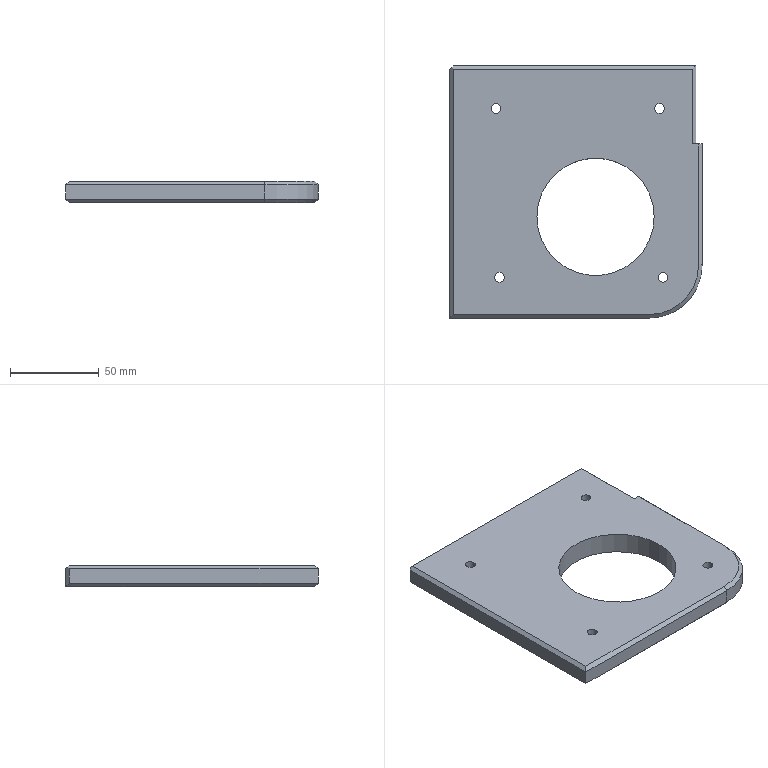Part | Creo | 1 solid | 43 faces | box 142 x 142 x 12 mm | volume 192544 mm3 | plane 22 | cylinder 19 | cone 2 | commonest cylinder face diameters 5.5 x8 9.5 x8 66 x2 60 x1
STEP:
#1=CARTESIAN_POINT('',(-313.,372.995,1.));
#2=VERTEX_POINT('',#1);
#3=CARTESIAN_POINT('',(-178.5,372.995,1.));
#4=VERTEX_POINT('',#3);
#5=CARTESIAN_POINT('',(-313.,372.995,1.));
#6=DIRECTION('',(1.,0.,0.));
#7=VECTOR('',#6,134.5);
#8=LINE('',#5,#7);
#9=EDGE_CURVE('',#2,#4,#8,.T.);
#10=ORIENTED_EDGE('',*,*,#9,.T.);
#11=CARTESIAN_POINT('',(-178.5,330.995,1.));
#12=VERTEX_POINT('',#11);
#13=CARTESIAN_POINT('',(-178.5,372.995,1.));
#14=DIRECTION('',(0.,-1.,0.));
#15=VECTOR('',#14,42.);
#16=LINE('',#13,#15);
#17=EDGE_CURVE('',#4,#12,#16,.T.);
#18=ORIENTED_EDGE('',*,*,#17,.T.);
#19=CARTESIAN_POINT('',(-175.,330.995,1.));
#20=VERTEX_POINT('',#19);
#21=CARTESIAN_POINT('',(-175.,330.995,1.));
#22=DIRECTION('',(-1.,0.,0.));
#23=VECTOR('',#22,3.5);
#24=LINE('',#21,#23);
#25=EDGE_CURVE('',#20,#12,#24,.T.);
#26=ORIENTED_EDGE('',*,*,#25,.F.);
#27=CARTESIAN_POINT('',(-175.,262.995,1.));
#28=VERTEX_POINT('',#27);
#29=CARTESIAN_POINT('',(-175.,330.995,1.));
#30=DIRECTION('',(0.,-1.,0.));
#31=VECTOR('',#30,68.);
#32=LINE('',#29,#31);
#33=EDGE_CURVE('',#20,#28,#32,.T.);
#34=ORIENTED_EDGE('',*,*,#33,.T.);
#35=CARTESIAN_POINT('',(-203.,234.995,1.));
#36=VERTEX_POINT('',#35);
#37=CARTESIAN_POINT('',(-203.,262.995,1.));
#38=DIRECTION('',(0.,0.,1.));
#39=DIRECTION('',(0.,-1.,0.));
#40=AXIS2_PLACEMENT_3D('',#37,#38,#39);
#41=CIRCLE('',#40,28.);
#42=EDGE_CURVE('',#36,#28,#41,.T.);
#43=ORIENTED_EDGE('',*,*,#42,.F.);
#44=CARTESIAN_POINT('',(-313.,234.995,1.));
#45=VERTEX_POINT('',#44);
#46=CARTESIAN_POINT('',(-203.,234.995,1.));
#47=DIRECTION('',(-1.,0.,0.));
#48=VECTOR('',#47,110.);
#49=LINE('',#46,#48);
#50=EDGE_CURVE('',#36,#45,#49,.T.);
#51=ORIENTED_EDGE('',*,*,#50,.T.);
#52=CARTESIAN_POINT('',(-313.,234.995,1.));
#53=DIRECTION('',(0.,1.,0.));
#54=VECTOR('',#53,138.);
#55=LINE('',#52,#54);
#56=EDGE_CURVE('',#45,#2,#55,.T.);
#57=ORIENTED_EDGE('',*,*,#56,.T.);
#58=EDGE_LOOP('',(#10,#18,#26,#34,#43,#51,#57));
#59=FACE_OUTER_BOUND('',#58,.F.);
#60=CARTESIAN_POINT('',(-197.75,256.,1.));
#61=VERTEX_POINT('',#60);
#62=CARTESIAN_POINT('',(-192.25,256.,1.));
#63=VERTEX_POINT('',#62);
#64=CARTESIAN_POINT('',(-195.,256.,1.));
#65=DIRECTION('',(0.,0.,-1.));
#66=DIRECTION('',(-1.,0.,0.));
#67=AXIS2_PLACEMENT_3D('',#64,#65,#66);
#68=CIRCLE('',#67,2.75);
#69=EDGE_CURVE('',#61,#63,#68,.T.);
#70=ORIENTED_EDGE('',*,*,#69,.F.);
#71=CARTESIAN_POINT('',(-195.,256.,1.));
#72=DIRECTION('',(0.,0.,-1.));
#73=DIRECTION('',(1.,0.,0.));
#74=AXIS2_PLACEMENT_3D('',#71,#72,#73);
#75=CIRCLE('',#74,2.75);
#76=EDGE_CURVE('',#63,#61,#75,.T.);
#77=ORIENTED_EDGE('',*,*,#76,.F.);
#78=EDGE_LOOP('',(#70,#77));
#79=FACE_BOUND('',#78,.F.);
#80=CARTESIAN_POINT('',(-289.75,256.,1.));
#81=VERTEX_POINT('',#80);
#82=CARTESIAN_POINT('',(-284.25,256.,1.));
#83=VERTEX_POINT('',#82);
#84=CARTESIAN_POINT('',(-287.,256.,1.));
#85=DIRECTION('',(0.,0.,-1.));
#86=DIRECTION('',(-1.,0.,0.));
#87=AXIS2_PLACEMENT_3D('',#84,#85,#86);
#88=CIRCLE('',#87,2.75);
#89=EDGE_CURVE('',#81,#83,#88,.T.);
#90=ORIENTED_EDGE('',*,*,#89,.F.);
#91=CARTESIAN_POINT('',(-287.,256.,1.));
#92=DIRECTION('',(0.,0.,-1.));
#93=DIRECTION('',(1.,0.,0.));
#94=AXIS2_PLACEMENT_3D('',#91,#92,#93);
#95=CIRCLE('',#94,2.75);
#96=EDGE_CURVE('',#83,#81,#95,.T.);
#97=ORIENTED_EDGE('',*,*,#96,.F.);
#98=EDGE_LOOP('',(#90,#97));
#99=FACE_BOUND('',#98,.F.);
#100=CARTESIAN_POINT('',(-200.,289.995,1.));
#101=VERTEX_POINT('',#100);
#102=CARTESIAN_POINT('',(-266.,289.995,1.));
#103=VERTEX_POINT('',#102);
#104=CARTESIAN_POINT('',(-233.,289.995,1.));
#105=DIRECTION('',(0.,0.,-1.));
#106=DIRECTION('',(1.,0.,0.));
#107=AXIS2_PLACEMENT_3D('',#104,#105,#106);
#108=CIRCLE('',#107,33.);
#109=EDGE_CURVE('',#101,#103,#108,.T.);
#110=ORIENTED_EDGE('',*,*,#109,.F.);
#111=CARTESIAN_POINT('',(-233.,289.995,1.));
#112=DIRECTION('',(0.,0.,-1.));
#113=DIRECTION('',(-1.,0.,0.));
#114=AXIS2_PLACEMENT_3D('',#111,#112,#113);
#115=CIRCLE('',#114,33.);
#116=EDGE_CURVE('',#103,#101,#115,.T.);
#117=ORIENTED_EDGE('',*,*,#116,.F.);
#118=EDGE_LOOP('',(#110,#117));
#119=FACE_BOUND('',#118,.F.);
#120=CARTESIAN_POINT('',(-199.699,351.,1.));
#121=VERTEX_POINT('',#120);
#122=CARTESIAN_POINT('',(-194.199,351.,1.));
#123=VERTEX_POINT('',#122);
#124=CARTESIAN_POINT('',(-196.949,351.,1.));
#125=DIRECTION('',(0.,0.,-1.));
#126=DIRECTION('',(-1.,0.,0.));
#127=AXIS2_PLACEMENT_3D('',#124,#125,#126);
#128=CIRCLE('',#127,2.75);
#129=EDGE_CURVE('',#121,#123,#128,.T.);
#130=ORIENTED_EDGE('',*,*,#129,.F.);
#131=CARTESIAN_POINT('',(-196.949,351.,1.));
#132=DIRECTION('',(0.,0.,-1.));
#133=DIRECTION('',(1.,0.,0.));
#134=AXIS2_PLACEMENT_3D('',#131,#132,#133);
#135=CIRCLE('',#134,2.75);
#136=EDGE_CURVE('',#123,#121,#135,.T.);
#137=ORIENTED_EDGE('',*,*,#136,.F.);
#138=EDGE_LOOP('',(#130,#137));
#139=FACE_BOUND('',#138,.F.);
#140=CARTESIAN_POINT('',(-291.699,351.,1.));
#141=VERTEX_POINT('',#140);
#142=CARTESIAN_POINT('',(-286.199,351.,1.));
#143=VERTEX_POINT('',#142);
#144=CARTESIAN_POINT('',(-288.949,351.,1.));
#145=DIRECTION('',(0.,0.,-1.));
#146=DIRECTION('',(-1.,0.,0.));
#147=AXIS2_PLACEMENT_3D('',#144,#145,#146);
#148=CIRCLE('',#147,2.75);
#149=EDGE_CURVE('',#141,#143,#148,.T.);
#150=ORIENTED_EDGE('',*,*,#149,.F.);
#151=CARTESIAN_POINT('',(-288.949,351.,1.));
#152=DIRECTION('',(0.,0.,-1.));
#153=DIRECTION('',(1.,0.,0.));
#154=AXIS2_PLACEMENT_3D('',#151,#152,#153);
#155=CIRCLE('',#154,2.75);
#156=EDGE_CURVE('',#143,#141,#155,.T.);
#157=ORIENTED_EDGE('',*,*,#156,.F.);
#158=EDGE_LOOP('',(#150,#157));
#159=FACE_BOUND('',#158,.F.);
#160=CARTESIAN_POINT('',(-223.,300.495,1.));
#161=DIRECTION('',(0.,0.,1.));
#162=DIRECTION('',(-1.,0.,0.));
#163=AXIS2_PLACEMENT_3D('',#160,#161,#162);
#164=PLANE('',#163);
#165=ADVANCED_FACE('',(#59,#79,#99,#119,#139,#159),#164,.T.);
#166=ORIENTED_EDGE('',*,*,#89,.T.);
#167=CARTESIAN_POINT('',(-284.25,256.,-5.));
#168=VERTEX_POINT('',#167);
#169=CARTESIAN_POINT('',(-284.25,256.,1.));
#170=DIRECTION('',(0.,0.,-1.));
#171=VECTOR('',#170,6.);
#172=LINE('',#169,#171);
#173=EDGE_CURVE('',#83,#168,#172,.T.);
#174=ORIENTED_EDGE('',*,*,#173,.T.);
#175=CARTESIAN_POINT('',(-289.75,256.,-5.));
#176=VERTEX_POINT('',#175);
#177=CARTESIAN_POINT('',(-287.,256.,-5.));
#178=DIRECTION('',(0.,0.,1.));
#179=DIRECTION('',(1.,0.,0.));
#180=AXIS2_PLACEMENT_3D('',#177,#178,#179);
#181=CIRCLE('',#180,2.75);
#182=EDGE_CURVE('',#168,#176,#181,.T.);
#183=ORIENTED_EDGE('',*,*,#182,.T.);
#184=CARTESIAN_POINT('',(-289.75,256.,1.));
#185=DIRECTION('',(0.,0.,-1.));
#186=VECTOR('',#185,6.);
#187=LINE('',#184,#186);
#188=EDGE_CURVE('',#81,#176,#187,.T.);
#189=ORIENTED_EDGE('',*,*,#188,.F.);
#190=EDGE_LOOP('',(#166,#174,#183,#189));
#191=FACE_OUTER_BOUND('',#190,.F.);
#192=CARTESIAN_POINT('',(-287.,256.,-11.));
#193=DIRECTION('',(0.,0.,-1.));
#194=DIRECTION('',(-1.,0.,0.));
#195=AXIS2_PLACEMENT_3D('',#192,#193,#194);
#196=CYLINDRICAL_SURFACE('',#195,2.75);
#197=ADVANCED_FACE('',(#191),#196,.F.);
#198=ORIENTED_EDGE('',*,*,#96,.T.);
#199=ORIENTED_EDGE('',*,*,#188,.T.);
#200=CARTESIAN_POINT('',(-287.,256.,-5.));
#201=DIRECTION('',(0.,0.,1.));
#202=DIRECTION('',(-1.,0.,0.));
#203=AXIS2_PLACEMENT_3D('',#200,#201,#202);
#204=CIRCLE('',#203,2.75);
#205=EDGE_CURVE('',#176,#168,#204,.T.);
#206=ORIENTED_EDGE('',*,*,#205,.T.);
#207=ORIENTED_EDGE('',*,*,#173,.F.);
#208=EDGE_LOOP('',(#198,#199,#206,#207));
#209=FACE_OUTER_BOUND('',#208,.F.);
#210=CARTESIAN_POINT('',(-287.,256.,-11.));
#211=DIRECTION('',(0.,0.,-1.));
#212=DIRECTION('',(-1.,0.,0.));
#213=AXIS2_PLACEMENT_3D('',#210,#211,#212);
#214=CYLINDRICAL_SURFACE('',#213,2.75);
#215=ADVANCED_FACE('',(#209),#214,.F.);
#216=CARTESIAN_POINT('',(-291.75,256.,-5.));
#217=VERTEX_POINT('',#216);
#218=CARTESIAN_POINT('',(-282.25,256.,-5.));
#219=VERTEX_POINT('',#218);
#220=CARTESIAN_POINT('',(-287.,256.,-5.));
#221=DIRECTION('',(0.,0.,-1.));
#222=DIRECTION('',(-1.,0.,0.));
#223=AXIS2_PLACEMENT_3D('',#220,#221,#222);
#224=CIRCLE('',#223,4.75);
#225=EDGE_CURVE('',#217,#219,#224,.T.);
#226=ORIENTED_EDGE('',*,*,#225,.F.);
#227=CARTESIAN_POINT('',(-287.,256.,-5.));
#228=DIRECTION('',(0.,0.,-1.));
#229=DIRECTION('',(1.,0.,0.));
#230=AXIS2_PLACEMENT_3D('',#227,#228,#229);
#231=CIRCLE('',#230,4.75);
#232=EDGE_CURVE('',#219,#217,#231,.T.);
#233=ORIENTED_EDGE('',*,*,#232,.F.);
#234=EDGE_LOOP('',(#226,#233));
#235=FACE_OUTER_BOUND('',#234,.F.);
#236=ORIENTED_EDGE('',*,*,#205,.F.);
#237=ORIENTED_EDGE('',*,*,#182,.F.);
#238=EDGE_LOOP('',(#236,#237));
#239=FACE_BOUND('',#238,.F.);
#240=CARTESIAN_POINT('',(-287.,260.75,-5.));
#241=DIRECTION('',(0.,0.,1.));
#242=DIRECTION('',(1.,0.,0.));
#243=AXIS2_PLACEMENT_3D('',#240,#241,#242);
#244=PLANE('',#243);
#245=ADVANCED_FACE('',(#235,#239),#244,.F.);
#246=ORIENTED_EDGE('',*,*,#225,.T.);
#247=CARTESIAN_POINT('',(-282.25,256.,-11.));
#248=VERTEX_POINT('',#247);
#249=CARTESIAN_POINT('',(-282.25,256.,-5.));
#250=DIRECTION('',(0.,0.,-1.));
#251=VECTOR('',#250,6.);
#252=LINE('',#249,#251);
#253=EDGE_CURVE('',#219,#248,#252,.T.);
#254=ORIENTED_EDGE('',*,*,#253,.T.);
#255=CARTESIAN_POINT('',(-291.75,256.,-11.));
#256=VERTEX_POINT('',#255);
#257=CARTESIAN_POINT('',(-287.,256.,-11.));
#258=DIRECTION('',(0.,0.,1.));
#259=DIRECTION('',(1.,0.,0.));
#260=AXIS2_PLACEMENT_3D('',#257,#258,#259);
#261=CIRCLE('',#260,4.75);
#262=EDGE_CURVE('',#248,#256,#261,.T.);
#263=ORIENTED_EDGE('',*,*,#262,.T.);
#264=CARTESIAN_POINT('',(-291.75,256.,-5.));
#265=DIRECTION('',(0.,0.,-1.));
#266=VECTOR('',#265,6.);
#267=LINE('',#264,#266);
#268=EDGE_CURVE('',#217,#256,#267,.T.);
#269=ORIENTED_EDGE('',*,*,#268,.F.);
#270=EDGE_LOOP('',(#246,#254,#263,#269));
#271=FACE_OUTER_BOUND('',#270,.F.);
#272=CARTESIAN_POINT('',(-287.,256.,-11.));
#273=DIRECTION('',(0.,0.,-1.));
#274=DIRECTION('',(-1.,0.,0.));
#275=AXIS2_PLACEMENT_3D('',#272,#273,#274);
#276=CYLINDRICAL_SURFACE('',#275,4.75);
#277=ADVANCED_FACE('',(#271),#276,.F.);
#278=ORIENTED_EDGE('',*,*,#232,.T.);
#279=ORIENTED_EDGE('',*,*,#268,.T.);
#280=CARTESIAN_POINT('',(-287.,256.,-11.));
#281=DIRECTION('',(0.,0.,1.));
#282=DIRECTION('',(-1.,0.,0.));
#283=AXIS2_PLACEMENT_3D('',#280,#281,#282);
#284=CIRCLE('',#283,4.75);
#285=EDGE_CURVE('',#256,#248,#284,.T.);
#286=ORIENTED_EDGE('',*,*,#285,.T.);
#287=ORIENTED_EDGE('',*,*,#253,.F.);
#288=EDGE_LOOP('',(#278,#279,#286,#287));
#289=FACE_OUTER_BOUND('',#288,.F.);
#290=CARTESIAN_POINT('',(-287.,256.,-11.));
#291=DIRECTION('',(0.,0.,-1.));
#292=DIRECTION('',(-1.,0.,0.));
#293=AXIS2_PLACEMENT_3D('',#290,#291,#292);
#294=CYLINDRICAL_SURFACE('',#293,4.75);
#295=ADVANCED_FACE('',(#289),#294,.F.);
#296=CARTESIAN_POINT('',(-313.,234.995,-11.));
#297=VERTEX_POINT('',#296);
#298=CARTESIAN_POINT('',(-203.,234.995,-11.));
#299=VERTEX_POINT('',#298);
#300=CARTESIAN_POINT('',(-313.,234.995,-11.));
#301=DIRECTION('',(1.,0.,0.));
#302=VECTOR('',#301,110.);
#303=LINE('',#300,#302);
#304=EDGE_CURVE('',#297,#299,#303,.T.);
#305=ORIENTED_EDGE('',*,*,#304,.T.);
#306=CARTESIAN_POINT('',(-175.,262.995,-11.));
#307=VERTEX_POINT('',#306);
#308=CARTESIAN_POINT('',(-203.,262.995,-11.));
#309=DIRECTION('',(0.,0.,-1.));
#310=DIRECTION('',(1.,0.,0.));
#311=AXIS2_PLACEMENT_3D('',#308,#309,#310);
#312=CIRCLE('',#311,28.);
#313=EDGE_CURVE('',#307,#299,#312,.T.);
#314=ORIENTED_EDGE('',*,*,#313,.F.);
#315=CARTESIAN_POINT('',(-175.,330.995,-11.));
#316=VERTEX_POINT('',#315);
#317=CARTESIAN_POINT('',(-175.,262.995,-11.));
#318=DIRECTION('',(0.,1.,0.));
#319=VECTOR('',#318,68.);
#320=LINE('',#317,#319);
#321=EDGE_CURVE('',#307,#316,#320,.T.);
#322=ORIENTED_EDGE('',*,*,#321,.T.);
#323=CARTESIAN_POINT('',(-178.5,330.995,-11.));
#324=VERTEX_POINT('',#323);
#325=CARTESIAN_POINT('',(-178.5,330.995,-11.));
#326=DIRECTION('',(1.,0.,0.));
#327=VECTOR('',#326,3.5);
#328=LINE('',#325,#327);
#329=EDGE_CURVE('',#324,#316,#328,.T.);
#330=ORIENTED_EDGE('',*,*,#329,.F.);
#331=CARTESIAN_POINT('',(-178.5,374.995,-11.));
#332=VERTEX_POINT('',#331);
#333=CARTESIAN_POINT('',(-178.5,330.995,-11.));
#334=DIRECTION('',(0.,1.,0.));
#335=VECTOR('',#334,44.);
#336=LINE('',#333,#335);
#337=EDGE_CURVE('',#324,#332,#336,.T.);
#338=ORIENTED_EDGE('',*,*,#337,.T.);
#339=CARTESIAN_POINT('',(-313.,374.995,-11.));
#340=VERTEX_POINT('',#339);
#341=CARTESIAN_POINT('',(-313.,374.995,-11.));
#342=DIRECTION('',(1.,0.,0.));
#343=VECTOR('',#342,134.5);
#344=LINE('',#341,#343);
#345=EDGE_CURVE('',#340,#332,#344,.T.);
#346=ORIENTED_EDGE('',*,*,#345,.F.);
#347=CARTESIAN_POINT('',(-313.,374.995,-11.));
#348=DIRECTION('',(0.,-1.,0.));
#349=VECTOR('',#348,140.);
#350=LINE('',#347,#349);
#351=EDGE_CURVE('',#340,#297,#350,.T.);
#352=ORIENTED_EDGE('',*,*,#351,.T.);
#353=EDGE_LOOP('',(#305,#314,#322,#330,#338,#346,#352));
#354=FACE_OUTER_BOUND('',#353,.F.);
#355=CARTESIAN_POINT('',(-293.699,351.,-11.));
#356=VERTEX_POINT('',#355);
#357=CARTESIAN_POINT('',(-284.199,351.,-11.));
#358=VERTEX_POINT('',#357);
#359=CARTESIAN_POINT('',(-288.949,351.,-11.));
#360=DIRECTION('',(0.,0.,1.));
#361=DIRECTION('',(-1.,0.,0.));
#362=AXIS2_PLACEMENT_3D('',#359,#360,#361);
#363=CIRCLE('',#362,4.75);
#364=EDGE_CURVE('',#356,#358,#363,.T.);
#365=ORIENTED_EDGE('',*,*,#364,.F.);
#366=CARTESIAN_POINT('',(-288.949,351.,-11.));
#367=DIRECTION('',(0.,0.,1.));
#368=DIRECTION('',(1.,0.,0.));
#369=AXIS2_PLACEMENT_3D('',#366,#367,#368);
#370=CIRCLE('',#369,4.75);
#371=EDGE_CURVE('',#358,#356,#370,.T.);
#372=ORIENTED_EDGE('',*,*,#371,.F.);
#373=EDGE_LOOP('',(#365,#372));
#374=FACE_BOUND('',#373,.F.);
#375=ORIENTED_EDGE('',*,*,#285,.F.);
#376=ORIENTED_EDGE('',*,*,#262,.F.);
#377=EDGE_LOOP('',(#375,#376));
#378=FACE_BOUND('',#377,.F.);
#379=CARTESIAN_POINT('',(-201.699,351.,-11.));
#380=VERTEX_POINT('',#379);
#381=CARTESIAN_POINT('',(-192.199,351.,-11.));
#382=VERTEX_POINT('',#381);
#383=CARTESIAN_POINT('',(-196.949,351.,-11.));
#384=DIRECTION('',(0.,0.,1.));
#385=DIRECTION('',(-1.,0.,0.));
#386=AXIS2_PLACEMENT_3D('',#383,#384,#385);
#387=CIRCLE('',#386,4.75);
#388=EDGE_CURVE('',#380,#382,#387,.T.);
#389=ORIENTED_EDGE('',*,*,#388,.F.);
#390=CARTESIAN_POINT('',(-196.949,351.,-11.));
#391=DIRECTION('',(0.,0.,1.));
#392=DIRECTION('',(1.,0.,0.));
#393=AXIS2_PLACEMENT_3D('',#390,#391,#392);
#394=CIRCLE('',#393,4.75);
#395=EDGE_CURVE('',#382,#380,#394,.T.);
#396=ORIENTED_EDGE('',*,*,#395,.F.);
#397=EDGE_LOOP('',(#389,#396));
#398=FACE_BOUND('',#397,.F.);
#399=CARTESIAN_POINT('',(-199.75,256.,-11.));
#400=VERTEX_POINT('',#399);
#401=CARTESIAN_POINT('',(-190.25,256.,-11.));
#402=VERTEX_POINT('',#401);
#403=CARTESIAN_POINT('',(-195.,256.,-11.));
#404=DIRECTION('',(0.,0.,1.));
#405=DIRECTION('',(-1.,0.,0.));
#406=AXIS2_PLACEMENT_3D('',#403,#404,#405);
#407=CIRCLE('',#406,4.75);
#408=EDGE_CURVE('',#400,#402,#407,.T.);
#409=ORIENTED_EDGE('',*,*,#408,.F.);
#410=CARTESIAN_POINT('',(-195.,256.,-11.));
#411=DIRECTION('',(0.,0.,1.));
#412=DIRECTION('',(1.,0.,0.));
#413=AXIS2_PLACEMENT_3D('',#410,#411,#412);
#414=CIRCLE('',#413,4.75);
#415=EDGE_CURVE('',#402,#400,#414,.T.);
#416=ORIENTED_EDGE('',*,*,#415,.F.);
#417=EDGE_LOOP('',(#409,#416));
#418=FACE_BOUND('',#417,.F.);
#419=CARTESIAN_POINT('',(-266.,289.995,-11.));
#420=VERTEX_POINT('',#419);
#421=CARTESIAN_POINT('',(-200.,289.995,-11.));
#422=VERTEX_POINT('',#421);
#423=CARTESIAN_POINT('',(-233.,289.995,-11.));
#424=DIRECTION('',(0.,0.,1.));
#425=DIRECTION('',(-1.,0.,0.));
#426=AXIS2_PLACEMENT_3D('',#423,#424,#425);
#427=CIRCLE('',#426,33.);
#428=EDGE_CURVE('',#420,#422,#427,.T.);
#429=ORIENTED_EDGE('',*,*,#428,.F.);
#430=CARTESIAN_POINT('',(-233.,289.995,-11.));
#431=DIRECTION('',(0.,0.,1.));
#432=DIRECTION('',(1.,0.,0.));
#433=AXIS2_PLACEMENT_3D('',#430,#431,#432);
#434=CIRCLE('',#433,33.);
#435=EDGE_CURVE('',#422,#420,#434,.T.);
#436=ORIENTED_EDGE('',*,*,#435,.F.);
#437=EDGE_LOOP('',(#429,#436));
#438=FACE_BOUND('',#437,.F.);
#439=CARTESIAN_POINT('',(-223.,300.495,-11.));
#440=DIRECTION('',(0.,0.,-1.));
#441=DIRECTION('',(1.,0.,0.));
#442=AXIS2_PLACEMENT_3D('',#439,#440,#441);
#443=PLANE('',#442);
#444=ADVANCED_FACE('',(#354,#374,#378,#398,#418,#438),#443,.T.);
#445=CARTESIAN_POINT('',(-203.,232.995,-9.));
#446=VERTEX_POINT('',#445);
#447=CARTESIAN_POINT('',(-315.,232.995,-9.));
#448=VERTEX_POINT('',#447);
#449=CARTESIAN_POINT('',(-203.,232.995,-9.));
#450=DIRECTION('',(-1.,0.,0.));
#451=VECTOR('',#450,112.);
#452=LINE('',#449,#451);
#453=EDGE_CURVE('',#446,#448,#452,.T.);
#454=ORIENTED_EDGE('',*,*,#453,.F.);
#455=CARTESIAN_POINT('',(-203.,232.995,-9.));
#456=DIRECTION('',(0.,0.7071,-0.7071));
#457=VECTOR('',#456,2.828);
#458=LINE('',#455,#457);
#459=EDGE_CURVE('',#446,#299,#458,.T.);
#460=ORIENTED_EDGE('',*,*,#459,.T.);
#461=ORIENTED_EDGE('',*,*,#304,.F.);
#462=CARTESIAN_POINT('',(-313.,234.995,-11.));
#463=DIRECTION('',(-0.5774,-0.5774,0.5774));
#464=VECTOR('',#463,3.464);
#465=LINE('',#462,#464);
#466=EDGE_CURVE('',#297,#448,#465,.T.);
#467=ORIENTED_EDGE('',*,*,#466,.T.);
#468=EDGE_LOOP('',(#454,#460,#461,#467));
#469=FACE_OUTER_BOUND('',#468,.F.);
#470=CARTESIAN_POINT('',(-223.,232.995,-9.));
#471=DIRECTION('',(0.,0.7071,0.7071));
#472=DIRECTION('',(1.,0.,0.));
#473=AXIS2_PLACEMENT_3D('',#470,#471,#472);
#474=PLANE('',#473);
#475=ADVANCED_FACE('',(#469),#474,.F.);
#476=CARTESIAN_POINT('',(-315.,232.995,-1.));
#477=VERTEX_POINT('',#476);
#478=CARTESIAN_POINT('',(-315.,232.995,-1.));
#479=DIRECTION('',(0.,0.,-1.));
#480=VECTOR('',#479,8.);
#481=LINE('',#478,#480);
#482=EDGE_CURVE('',#477,#448,#481,.T.);
#483=ORIENTED_EDGE('',*,*,#482,.F.);
#484=CARTESIAN_POINT('',(-203.,232.995,-1.));
#485=VERTEX_POINT('',#484);
#486=CARTESIAN_POINT('',(-315.,232.995,-1.));
#487=DIRECTION('',(1.,0.,0.));
#488=VECTOR('',#487,112.);
#489=LINE('',#486,#488);
#490=EDGE_CURVE('',#477,#485,#489,.T.);
#491=ORIENTED_EDGE('',*,*,#490,.T.);
#492=CARTESIAN_POINT('',(-203.,232.995,-1.));
#493=DIRECTION('',(0.,0.,-1.));
#494=VECTOR('',#493,8.);
#495=LINE('',#492,#494);
#496=EDGE_CURVE('',#485,#446,#495,.T.);
#497=ORIENTED_EDGE('',*,*,#496,.T.);
#498=ORIENTED_EDGE('',*,*,#453,.T.);
#499=EDGE_LOOP('',(#483,#491,#497,#498));
#500=FACE_OUTER_BOUND('',#499,.F.);
#501=CARTESIAN_POINT('',(-223.,232.995,-10.));
#502=DIRECTION('',(0.,-1.,0.));
#503=DIRECTION('',(0.,0.,1.));
#504=AXIS2_PLACEMENT_3D('',#501,#502,#503);
#505=PLANE('',#504);
#506=ADVANCED_FACE('',(#500),#505,.T.);
#507=CARTESIAN_POINT('',(-315.,372.995,-9.));
#508=VERTEX_POINT('',#507);
#509=CARTESIAN_POINT('',(-315.,372.995,-1.));
#510=VERTEX_POINT('',#509);
#511=CARTESIAN_POINT('',(-315.,372.995,-9.));
#512=DIRECTION('',(0.,0.,1.));
#513=VECTOR('',#512,8.);
#514=LINE('',#511,#513);
#515=EDGE_CURVE('',#508,#510,#514,.T.);
#516=ORIENTED_EDGE('',*,*,#515,.T.);
#517=CARTESIAN_POINT('',(-315.,372.995,-1.));
#518=DIRECTION('',(0.,-1.,0.));
#519=VECTOR('',#518,140.);
#520=LINE('',#517,#519);
#521=EDGE_CURVE('',#510,#477,#520,.T.);
#522=ORIENTED_EDGE('',*,*,#521,.T.);
#523=ORIENTED_EDGE('',*,*,#482,.T.);
#524=CARTESIAN_POINT('',(-315.,232.995,-9.));
#525=DIRECTION('',(0.,1.,0.));
#526=VECTOR('',#525,140.);
#527=LINE('',#524,#526);
#528=EDGE_CURVE('',#448,#508,#527,.T.);
#529=ORIENTED_EDGE('',*,*,#528,.T.);
#530=EDGE_LOOP('',(#516,#522,#523,#529));
#531=FACE_OUTER_BOUND('',#530,.F.);
#532=CARTESIAN_POINT('',(-315.,-0.004699,-1.));
#533=DIRECTION('',(1.,0.,0.));
#534=DIRECTION('',(0.,-1.,0.));
#535=AXIS2_PLACEMENT_3D('',#532,#533,#534);
#536=PLANE('',#535);
#537=ADVANCED_FACE('',(#531),#536,.F.);
#538=CARTESIAN_POINT('',(-313.,374.995,-1.));
#539=VERTEX_POINT('',#538);
#540=CARTESIAN_POINT('',(-313.,374.995,-1.));
#541=DIRECTION('',(0.,0.,-1.));
#542=VECTOR('',#541,10.);
#543=LINE('',#540,#542);
#544=EDGE_CURVE('',#539,#340,#543,.T.);
#545=ORIENTED_EDGE('',*,*,#544,.F.);
#546=CARTESIAN_POINT('',(-314.,373.995,0.));
#547=VERTEX_POINT('',#546);
#548=CARTESIAN_POINT('',(-313.,374.995,-1.));
#549=DIRECTION('',(-0.5774,-0.5774,0.5774));
#550=VECTOR('',#549,1.732);
#551=LINE('',#548,#550);
#552=EDGE_CURVE('',#539,#547,#551,.T.);
#553=ORIENTED_EDGE('',*,*,#552,.T.);
#554=CARTESIAN_POINT('',(-314.,373.995,0.));
#555=DIRECTION('',(-0.5774,-0.5774,-0.5774));
#556=VECTOR('',#555,1.732);
#557=LINE('',#554,#556);
#558=EDGE_CURVE('',#547,#510,#557,.T.);
#559=ORIENTED_EDGE('',*,*,#558,.T.);
#560=ORIENTED_EDGE('',*,*,#515,.F.);
#561=CARTESIAN_POINT('',(-315.,372.995,-9.));
#562=DIRECTION('',(0.5774,0.5774,-0.5774));
#563=VECTOR('',#562,3.464);
#564=LINE('',#561,#563);
#565=EDGE_CURVE('',#508,#340,#564,.T.);
#566=ORIENTED_EDGE('',*,*,#565,.T.);
#567=EDGE_LOOP('',(#545,#553,#559,#560,#566));
#568=FACE_OUTER_BOUND('',#567,.F.);
#569=CARTESIAN_POINT('',(-313.,374.995,-1.));
#570=DIRECTION('',(-0.7071,0.7071,0.));
#571=DIRECTION('',(0.,0.,-1.));
#572=AXIS2_PLACEMENT_3D('',#569,#570,#571);
#573=PLANE('',#572);
#574=ADVANCED_FACE('',(#568),#573,.T.);
#575=ORIENTED_EDGE('',*,*,#544,.T.);
#576=ORIENTED_EDGE('',*,*,#345,.T.);
#577=CARTESIAN_POINT('',(-176.5,374.995,-9.));
#578=VERTEX_POINT('',#577);
#579=CARTESIAN_POINT('',(-176.5,374.995,-9.));
#580=DIRECTION('',(-0.7071,0.,-0.7071));
#581=VECTOR('',#580,2.828);
#582=LINE('',#579,#581);
#583=EDGE_CURVE('',#578,#332,#582,.T.);
#584=ORIENTED_EDGE('',*,*,#583,.F.);
#585=CARTESIAN_POINT('',(-176.5,374.995,-1.));
#586=VERTEX_POINT('',#585);
#587=CARTESIAN_POINT('',(-176.5,374.995,-1.));
#588=DIRECTION('',(0.,0.,-1.));
#589=VECTOR('',#588,8.);
#590=LINE('',#587,#589);
#591=EDGE_CURVE('',#586,#578,#590,.T.);
#592=ORIENTED_EDGE('',*,*,#591,.F.);
#593=CARTESIAN_POINT('',(-176.5,374.995,-1.));
#594=DIRECTION('',(-1.,0.,0.));
#595=VECTOR('',#594,136.5);
#596=LINE('',#593,#595);
#597=EDGE_CURVE('',#586,#539,#596,.T.);
#598=ORIENTED_EDGE('',*,*,#597,.T.);
#599=EDGE_LOOP('',(#575,#576,#584,#592,#598));
#600=FACE_OUTER_BOUND('',#599,.F.);
#601=CARTESIAN_POINT('',(-265.,374.995,-1.));
#602=DIRECTION('',(0.,1.,0.));
#603=DIRECTION('',(0.,0.,1.));
#604=AXIS2_PLACEMENT_3D('',#601,#602,#603);
#605=PLANE('',#604);
#606=ADVANCED_FACE('',(#600),#605,.T.);
#607=CARTESIAN_POINT('',(-176.5,330.995,-9.));
#608=VERTEX_POINT('',#607);
#609=CARTESIAN_POINT('',(-178.5,330.995,-11.));
#610=DIRECTION('',(0.7071,0.,0.7071));
#611=VECTOR('',#610,2.828);
#612=LINE('',#609,#611);
#613=EDGE_CURVE('',#324,#608,#612,.T.);
#614=ORIENTED_EDGE('',*,*,#613,.T.);
#615=CARTESIAN_POINT('',(-176.5,374.995,-9.));
#616=DIRECTION('',(0.,-1.,0.));
#617=VECTOR('',#616,44.);
#618=LINE('',#615,#617);
#619=EDGE_CURVE('',#578,#608,#618,.T.);
#620=ORIENTED_EDGE('',*,*,#619,.F.);
#621=ORIENTED_EDGE('',*,*,#583,.T.);
#622=ORIENTED_EDGE('',*,*,#337,.F.);
#623=EDGE_LOOP('',(#614,#620,#621,#622));
#624=FACE_OUTER_BOUND('',#623,.F.);
#625=CARTESIAN_POINT('',(-176.5,393.995,-9.));
#626=DIRECTION('',(0.7071,0.,-0.7071));
#627=DIRECTION('',(0.,-1.,0.));
#628=AXIS2_PLACEMENT_3D('',#625,#626,#627);
#629=PLANE('',#628);
#630=ADVANCED_FACE('',(#624),#629,.T.);
#631=CARTESIAN_POINT('',(-173.,330.995,-9.));
#632=VERTEX_POINT('',#631);
#633=CARTESIAN_POINT('',(-173.,330.995,-1.));
#634=VERTEX_POINT('',#633);
#635=CARTESIAN_POINT('',(-173.,330.995,-9.));
#636=DIRECTION('',(0.,0.,1.));
#637=VECTOR('',#636,8.);
#638=LINE('',#635,#637);
#639=EDGE_CURVE('',#632,#634,#638,.T.);
#640=ORIENTED_EDGE('',*,*,#639,.T.);
#641=CARTESIAN_POINT('',(-175.,330.995,1.));
#642=DIRECTION('',(0.7071,0.,-0.7071));
#643=VECTOR('',#642,2.828);
#644=LINE('',#641,#643);
#645=EDGE_CURVE('',#20,#634,#644,.T.);
#646=ORIENTED_EDGE('',*,*,#645,.F.);
#647=ORIENTED_EDGE('',*,*,#25,.T.);
#648=CARTESIAN_POINT('',(-176.5,330.995,-1.));
#649=VERTEX_POINT('',#648);
#650=CARTESIAN_POINT('',(-176.5,330.995,-1.));
#651=DIRECTION('',(-0.7071,0.,0.7071));
#652=VECTOR('',#651,2.828);
#653=LINE('',#650,#652);
#654=EDGE_CURVE('',#649,#12,#653,.T.);
#655=ORIENTED_EDGE('',*,*,#654,.F.);
#656=CARTESIAN_POINT('',(-176.5,330.995,-9.));
#657=DIRECTION('',(0.,0.,1.));
#658=VECTOR('',#657,8.);
#659=LINE('',#656,#658);
#660=EDGE_CURVE('',#608,#649,#659,.T.);
#661=ORIENTED_EDGE('',*,*,#660,.F.);
#662=ORIENTED_EDGE('',*,*,#613,.F.);
#663=ORIENTED_EDGE('',*,*,#329,.T.);
#664=CARTESIAN_POINT('',(-173.,330.995,-9.));
#665=DIRECTION('',(-0.7071,0.,-0.7071));
#666=VECTOR('',#665,2.828);
#667=LINE('',#664,#666);
#668=EDGE_CURVE('',#632,#316,#667,.T.);
#669=ORIENTED_EDGE('',*,*,#668,.F.);
#670=EDGE_LOOP('',(#640,#646,#647,#655,#661,#662,#663,#669));
#671=FACE_OUTER_BOUND('',#670,.F.);
#672=CARTESIAN_POINT('',(-155.,330.995,-21.));
#673=DIRECTION('',(0.,1.,0.));
#674=DIRECTION('',(-1.,0.,0.));
#675=AXIS2_PLACEMENT_3D('',#672,#673,#674);
#676=PLANE('',#675);
#677=ADVANCED_FACE('',(#671),#676,.T.);
#678=CARTESIAN_POINT('',(-173.,262.995,-9.));
#679=VERTEX_POINT('',#678);
#680=CARTESIAN_POINT('',(-173.,262.995,-1.));
#681=VERTEX_POINT('',#680);
#682=CARTESIAN_POINT('',(-173.,262.995,-9.));
#683=DIRECTION('',(0.,0.,1.));
#684=VECTOR('',#683,8.);
#685=LINE('',#682,#684);
#686=EDGE_CURVE('',#679,#681,#685,.T.);
#687=ORIENTED_EDGE('',*,*,#686,.T.);
#688=CARTESIAN_POINT('',(-173.,262.995,-1.));
#689=DIRECTION('',(0.,1.,0.));
#690=VECTOR('',#689,68.);
#691=LINE('',#688,#690);
#692=EDGE_CURVE('',#681,#634,#691,.T.);
#693=ORIENTED_EDGE('',*,*,#692,.T.);
#694=ORIENTED_EDGE('',*,*,#639,.F.);
#695=CARTESIAN_POINT('',(-173.,330.995,-9.));
#696=DIRECTION('',(0.,-1.,0.));
#697=VECTOR('',#696,68.);
#698=LINE('',#695,#697);
#699=EDGE_CURVE('',#632,#679,#698,.T.);
#700=ORIENTED_EDGE('',*,*,#699,.T.);
#701=EDGE_LOOP('',(#687,#693,#694,#700));
#702=FACE_OUTER_BOUND('',#701,.F.);
#703=CARTESIAN_POINT('',(-173.,-2.005,1.));
#704=DIRECTION('',(-1.,0.,0.));
#705=DIRECTION('',(0.,1.,0.));
#706=AXIS2_PLACEMENT_3D('',#703,#704,#705);
#707=PLANE('',#706);
#708=ADVANCED_FACE('',(#702),#707,.F.);
#709=ORIENTED_EDGE('',*,*,#496,.F.);
#710=CARTESIAN_POINT('',(-203.,262.995,-1.));
#711=DIRECTION('',(0.,0.,1.));
#712=DIRECTION('',(0.,-1.,0.));
#713=AXIS2_PLACEMENT_3D('',#710,#711,#712);
#714=CIRCLE('',#713,30.);
#715=EDGE_CURVE('',#485,#681,#714,.T.);
#716=ORIENTED_EDGE('',*,*,#715,.T.);
#717=ORIENTED_EDGE('',*,*,#686,.F.);
#718=CARTESIAN_POINT('',(-203.,262.995,-9.));
#719=DIRECTION('',(0.,0.,-1.));
#720=DIRECTION('',(1.,0.,0.));
#721=AXIS2_PLACEMENT_3D('',#718,#719,#720);
#722=CIRCLE('',#721,30.);
#723=EDGE_CURVE('',#679,#446,#722,.T.);
#724=ORIENTED_EDGE('',*,*,#723,.T.);
#725=EDGE_LOOP('',(#709,#716,#717,#724));
#726=FACE_OUTER_BOUND('',#725,.F.);
#727=CARTESIAN_POINT('',(-203.,262.995,-10.));
#728=DIRECTION('',(0.,0.,-1.));
#729=DIRECTION('',(1.,0.,0.));
#730=AXIS2_PLACEMENT_3D('',#727,#728,#729);
#731=CYLINDRICAL_SURFACE('',#730,30.);
#732=ADVANCED_FACE('',(#726),#731,.T.);
#733=CARTESIAN_POINT('',(-203.,234.995,1.));
#734=DIRECTION('',(0.,-0.7071,-0.7071));
#735=VECTOR('',#734,2.828);
#736=LINE('',#733,#735);
#737=EDGE_CURVE('',#36,#485,#736,.T.);
#738=ORIENTED_EDGE('',*,*,#737,.F.);
#739=ORIENTED_EDGE('',*,*,#42,.T.);
#740=CARTESIAN_POINT('',(-173.,262.995,-1.));
#741=DIRECTION('',(-0.7071,0.,0.7071));
#742=VECTOR('',#741,2.828);
#743=LINE('',#740,#742);
#744=EDGE_CURVE('',#681,#28,#743,.T.);
#745=ORIENTED_EDGE('',*,*,#744,.F.);
#746=ORIENTED_EDGE('',*,*,#715,.F.);
#747=EDGE_LOOP('',(#738,#739,#745,#746));
#748=FACE_OUTER_BOUND('',#747,.F.);
#749=CARTESIAN_POINT('',(-203.,262.995,0.));
#750=DIRECTION('',(0.,0.,-1.));
#751=DIRECTION('',(-1.,0.,0.));
#752=AXIS2_PLACEMENT_3D('',#749,#750,#751);
#753=CONICAL_SURFACE('',#752,29.,45.);
#754=ADVANCED_FACE('',(#748),#753,.T.);
#755=ORIENTED_EDGE('',*,*,#50,.F.);
#756=ORIENTED_EDGE('',*,*,#737,.T.);
#757=ORIENTED_EDGE('',*,*,#490,.F.);
#758=CARTESIAN_POINT('',(-315.,232.995,-1.));
#759=DIRECTION('',(0.5774,0.5774,0.5774));
#760=VECTOR('',#759,3.464);
#761=LINE('',#758,#760);
#762=EDGE_CURVE('',#477,#45,#761,.T.);
#763=ORIENTED_EDGE('',*,*,#762,.T.);
#764=EDGE_LOOP('',(#755,#756,#757,#763));
#765=FACE_OUTER_BOUND('',#764,.F.);
#766=CARTESIAN_POINT('',(-223.,232.995,-1.));
#767=DIRECTION('',(0.,0.7071,-0.7071));
#768=DIRECTION('',(-1.,0.,0.));
#769=AXIS2_PLACEMENT_3D('',#766,#767,#768);
#770=PLANE('',#769);
#771=ADVANCED_FACE('',(#765),#770,.F.);
#772=ORIENTED_EDGE('',*,*,#762,.F.);
#773=ORIENTED_EDGE('',*,*,#521,.F.);
#774=ORIENTED_EDGE('',*,*,#558,.F.);
#775=CARTESIAN_POINT('',(-314.,373.995,0.));
#776=DIRECTION('',(0.5774,-0.5774,0.5774));
#777=VECTOR('',#776,1.732);
#778=LINE('',#775,#777);
#779=EDGE_CURVE('',#547,#2,#778,.T.);
#780=ORIENTED_EDGE('',*,*,#779,.T.);
#781=ORIENTED_EDGE('',*,*,#56,.F.);
#782=EDGE_LOOP('',(#772,#773,#774,#780,#781));
#783=FACE_OUTER_BOUND('',#782,.F.);
#784=CARTESIAN_POINT('',(-315.,-0.004699,-1.));
#785=DIRECTION('',(-0.7071,0.,0.7071));
#786=DIRECTION('',(0.,-1.,0.));
#787=AXIS2_PLACEMENT_3D('',#784,#785,#786);
#788=PLANE('',#787);
#789=ADVANCED_FACE('',(#783),#788,.T.);
#790=ORIENTED_EDGE('',*,*,#597,.F.);
#791=CARTESIAN_POINT('',(-176.5,374.995,-1.));
#792=DIRECTION('',(-0.5774,-0.5774,0.5774));
#793=VECTOR('',#792,3.464);
#794=LINE('',#791,#793);
#795=EDGE_CURVE('',#586,#4,#794,.T.);
#796=ORIENTED_EDGE('',*,*,#795,.T.);
#797=ORIENTED_EDGE('',*,*,#9,.F.);
#798=ORIENTED_EDGE('',*,*,#779,.F.);
#799=ORIENTED_EDGE('',*,*,#552,.F.);
#800=EDGE_LOOP('',(#790,#796,#797,#798,#799));
#801=FACE_OUTER_BOUND('',#800,.F.);
#802=CARTESIAN_POINT('',(-265.,374.995,-1.));
#803=DIRECTION('',(0.,-0.7071,-0.7071));
#804=DIRECTION('',(1.,0.,0.));
#805=AXIS2_PLACEMENT_3D('',#802,#803,#804);
#806=PLANE('',#805);
#807=ADVANCED_FACE('',(#801),#806,.F.);
#808=ORIENTED_EDGE('',*,*,#654,.T.);
#809=ORIENTED_EDGE('',*,*,#17,.F.);
#810=ORIENTED_EDGE('',*,*,#795,.F.);
#811=CARTESIAN_POINT('',(-176.5,330.995,-1.));
#812=DIRECTION('',(0.,1.,0.));
#813=VECTOR('',#812,44.);
#814=LINE('',#811,#813);
#815=EDGE_CURVE('',#649,#586,#814,.T.);
#816=ORIENTED_EDGE('',*,*,#815,.F.);
#817=EDGE_LOOP('',(#808,#809,#810,#816));
#818=FACE_OUTER_BOUND('',#817,.F.);
#819=CARTESIAN_POINT('',(-176.5,393.995,-1.));
#820=DIRECTION('',(0.7071,0.,0.7071));
#821=DIRECTION('',(0.,1.,0.));
#822=AXIS2_PLACEMENT_3D('',#819,#820,#821);
#823=PLANE('',#822);
#824=ADVANCED_FACE('',(#818),#823,.T.);
#825=ORIENTED_EDGE('',*,*,#591,.T.);
#826=ORIENTED_EDGE('',*,*,#619,.T.);
#827=ORIENTED_EDGE('',*,*,#660,.T.);
#828=ORIENTED_EDGE('',*,*,#815,.T.);
#829=EDGE_LOOP('',(#825,#826,#827,#828));
#830=FACE_OUTER_BOUND('',#829,.F.);
#831=CARTESIAN_POINT('',(-176.5,393.995,-195.076));
#832=DIRECTION('',(-1.,0.,0.));
#833=DIRECTION('',(0.,0.,1.));
#834=AXIS2_PLACEMENT_3D('',#831,#832,#833);
#835=PLANE('',#834);
#836=ADVANCED_FACE('',(#830),#835,.F.);
#837=ORIENTED_EDGE('',*,*,#645,.T.);
#838=ORIENTED_EDGE('',*,*,#692,.F.);
#839=ORIENTED_EDGE('',*,*,#744,.T.);
#840=ORIENTED_EDGE('',*,*,#33,.F.);
#841=EDGE_LOOP('',(#837,#838,#839,#840));
#842=FACE_OUTER_BOUND('',#841,.F.);
#843=CARTESIAN_POINT('',(-173.,-2.005,-1.));
#844=DIRECTION('',(0.7071,0.,0.7071));
#845=DIRECTION('',(0.,1.,0.));
#846=AXIS2_PLACEMENT_3D('',#843,#844,#845);
#847=PLANE('',#846);
#848=ADVANCED_FACE('',(#842),#847,.T.);
#849=ORIENTED_EDGE('',*,*,#459,.F.);
#850=ORIENTED_EDGE('',*,*,#723,.F.);
#851=CARTESIAN_POINT('',(-175.,262.995,-11.));
#852=DIRECTION('',(0.7071,0.,0.7071));
#853=VECTOR('',#852,2.828);
#854=LINE('',#851,#853);
#855=EDGE_CURVE('',#307,#679,#854,.T.);
#856=ORIENTED_EDGE('',*,*,#855,.F.);
#857=ORIENTED_EDGE('',*,*,#313,.T.);
#858=EDGE_LOOP('',(#849,#850,#856,#857));
#859=FACE_OUTER_BOUND('',#858,.F.);
#860=CARTESIAN_POINT('',(-203.,262.995,-10.));
#861=DIRECTION('',(0.,0.,1.));
#862=DIRECTION('',(1.,0.,0.));
#863=AXIS2_PLACEMENT_3D('',#860,#861,#862);
#864=CONICAL_SURFACE('',#863,29.,45.);
#865=ADVANCED_FACE('',(#859),#864,.T.);
#866=ORIENTED_EDGE('',*,*,#855,.T.);
#867=ORIENTED_EDGE('',*,*,#699,.F.);
#868=ORIENTED_EDGE('',*,*,#668,.T.);
#869=ORIENTED_EDGE('',*,*,#321,.F.);
#870=EDGE_LOOP('',(#866,#867,#868,#869));
#871=FACE_OUTER_BOUND('',#870,.F.);
#872=CARTESIAN_POINT('',(-173.,-2.005,-9.));
#873=DIRECTION('',(0.7071,0.,-0.7071));
#874=DIRECTION('',(0.,-1.,0.));
#875=AXIS2_PLACEMENT_3D('',#872,#873,#874);
#876=PLANE('',#875);
#877=ADVANCED_FACE('',(#871),#876,.T.);
#878=ORIENTED_EDGE('',*,*,#565,.F.);
#879=ORIENTED_EDGE('',*,*,#528,.F.);
#880=ORIENTED_EDGE('',*,*,#466,.F.);
#881=ORIENTED_EDGE('',*,*,#351,.F.);
#882=EDGE_LOOP('',(#878,#879,#880,#881));
#883=FACE_OUTER_BOUND('',#882,.F.);
#884=CARTESIAN_POINT('',(-315.,-0.004699,-9.));
#885=DIRECTION('',(-0.7071,0.,-0.7071));
#886=DIRECTION('',(0.,1.,0.));
#887=AXIS2_PLACEMENT_3D('',#884,#885,#886);
#888=PLANE('',#887);
#889=ADVANCED_FACE('',(#883),#888,.T.);
#890=CARTESIAN_POINT('',(-284.199,351.,-5.));
#891=VERTEX_POINT('',#890);
#892=CARTESIAN_POINT('',(-293.699,351.,-5.));
#893=VERTEX_POINT('',#892);
#894=CARTESIAN_POINT('',(-288.949,351.,-5.));
#895=DIRECTION('',(0.,0.,-1.));
#896=DIRECTION('',(1.,0.,0.));
#897=AXIS2_PLACEMENT_3D('',#894,#895,#896);
#898=CIRCLE('',#897,4.75);
#899=EDGE_CURVE('',#891,#893,#898,.T.);
#900=ORIENTED_EDGE('',*,*,#899,.T.);
#901=CARTESIAN_POINT('',(-293.699,351.,-5.));
#902=DIRECTION('',(0.,0.,-1.));
#903=VECTOR('',#902,6.);
#904=LINE('',#901,#903);
#905=EDGE_CURVE('',#893,#356,#904,.T.);
#906=ORIENTED_EDGE('',*,*,#905,.T.);
#907=ORIENTED_EDGE('',*,*,#364,.T.);
#908=CARTESIAN_POINT('',(-284.199,351.,-5.));
#909=DIRECTION('',(0.,0.,-1.));
#910=VECTOR('',#909,6.);
#911=LINE('',#908,#910);
#912=EDGE_CURVE('',#891,#358,#911,.T.);
#913=ORIENTED_EDGE('',*,*,#912,.F.);
#914=EDGE_LOOP('',(#900,#906,#907,#913));
#915=FACE_OUTER_BOUND('',#914,.F.);
#916=CARTESIAN_POINT('',(-288.949,351.,-11.));
#917=DIRECTION('',(0.,0.,-1.));
#918=DIRECTION('',(-1.,0.,0.));
#919=AXIS2_PLACEMENT_3D('',#916,#917,#918);
#920=CYLINDRICAL_SURFACE('',#919,4.75);
#921=ADVANCED_FACE('',(#915),#920,.F.);
#922=CARTESIAN_POINT('',(-288.949,351.,-5.));
#923=DIRECTION('',(0.,0.,-1.));
#924=DIRECTION('',(-1.,0.,0.));
#925=AXIS2_PLACEMENT_3D('',#922,#923,#924);
#926=CIRCLE('',#925,4.75);
#927=EDGE_CURVE('',#893,#891,#926,.T.);
#928=ORIENTED_EDGE('',*,*,#927,.F.);
#929=ORIENTED_EDGE('',*,*,#899,.F.);
#930=EDGE_LOOP('',(#928,#929));
#931=FACE_OUTER_BOUND('',#930,.F.);
#932=CARTESIAN_POINT('',(-291.699,351.,-5.));
#933=VERTEX_POINT('',#932);
#934=CARTESIAN_POINT('',(-286.199,351.,-5.));
#935=VERTEX_POINT('',#934);
#936=CARTESIAN_POINT('',(-288.949,351.,-5.));
#937=DIRECTION('',(0.,0.,1.));
#938=DIRECTION('',(-1.,0.,0.));
#939=AXIS2_PLACEMENT_3D('',#936,#937,#938);
#940=CIRCLE('',#939,2.75);
#941=EDGE_CURVE('',#933,#935,#940,.T.);
#942=ORIENTED_EDGE('',*,*,#941,.F.);
#943=CARTESIAN_POINT('',(-288.949,351.,-5.));
#944=DIRECTION('',(0.,0.,1.));
#945=DIRECTION('',(1.,0.,0.));
#946=AXIS2_PLACEMENT_3D('',#943,#944,#945);
#947=CIRCLE('',#946,2.75);
#948=EDGE_CURVE('',#935,#933,#947,.T.);
#949=ORIENTED_EDGE('',*,*,#948,.F.);
#950=EDGE_LOOP('',(#942,#949));
#951=FACE_BOUND('',#950,.F.);
#952=CARTESIAN_POINT('',(-288.949,355.75,-5.));
#953=DIRECTION('',(0.,0.,1.));
#954=DIRECTION('',(1.,0.,0.));
#955=AXIS2_PLACEMENT_3D('',#952,#953,#954);
#956=PLANE('',#955);
#957=ADVANCED_FACE('',(#931,#951),#956,.F.);
#958=ORIENTED_EDGE('',*,*,#156,.T.);
#959=CARTESIAN_POINT('',(-291.699,351.,1.));
#960=DIRECTION('',(0.,0.,-1.));
#961=VECTOR('',#960,6.);
#962=LINE('',#959,#961);
#963=EDGE_CURVE('',#141,#933,#962,.T.);
#964=ORIENTED_EDGE('',*,*,#963,.T.);
#965=ORIENTED_EDGE('',*,*,#941,.T.);
#966=CARTESIAN_POINT('',(-286.199,351.,1.));
#967=DIRECTION('',(0.,0.,-1.));
#968=VECTOR('',#967,6.);
#969=LINE('',#966,#968);
#970=EDGE_CURVE('',#143,#935,#969,.T.);
#971=ORIENTED_EDGE('',*,*,#970,.F.);
#972=EDGE_LOOP('',(#958,#964,#965,#971));
#973=FACE_OUTER_BOUND('',#972,.F.);
#974=CARTESIAN_POINT('',(-288.949,351.,-11.));
#975=DIRECTION('',(0.,0.,-1.));
#976=DIRECTION('',(-1.,0.,0.));
#977=AXIS2_PLACEMENT_3D('',#974,#975,#976);
#978=CYLINDRICAL_SURFACE('',#977,2.75);
#979=ADVANCED_FACE('',(#973),#978,.F.);
#980=ORIENTED_EDGE('',*,*,#149,.T.);
#981=ORIENTED_EDGE('',*,*,#970,.T.);
#982=ORIENTED_EDGE('',*,*,#948,.T.);
#983=ORIENTED_EDGE('',*,*,#963,.F.);
#984=EDGE_LOOP('',(#980,#981,#982,#983));
#985=FACE_OUTER_BOUND('',#984,.F.);
#986=CARTESIAN_POINT('',(-288.949,351.,-11.));
#987=DIRECTION('',(0.,0.,-1.));
#988=DIRECTION('',(-1.,0.,0.));
#989=AXIS2_PLACEMENT_3D('',#986,#987,#988);
#990=CYLINDRICAL_SURFACE('',#989,2.75);
#991=ADVANCED_FACE('',(#985),#990,.F.);
#992=ORIENTED_EDGE('',*,*,#927,.T.);
#993=ORIENTED_EDGE('',*,*,#912,.T.);
#994=ORIENTED_EDGE('',*,*,#371,.T.);
#995=ORIENTED_EDGE('',*,*,#905,.F.);
#996=EDGE_LOOP('',(#992,#993,#994,#995));
#997=FACE_OUTER_BOUND('',#996,.F.);
#998=CARTESIAN_POINT('',(-288.949,351.,-11.));
#999=DIRECTION('',(0.,0.,-1.));
#1000=DIRECTION('',(-1.,0.,0.));
#1001=AXIS2_PLACEMENT_3D('',#998,#999,#1000);
#1002=CYLINDRICAL_SURFACE('',#1001,4.75);
#1003=ADVANCED_FACE('',(#997),#1002,.F.);
#1004=CARTESIAN_POINT('',(-192.199,351.,-5.));
#1005=VERTEX_POINT('',#1004);
#1006=CARTESIAN_POINT('',(-201.699,351.,-5.));
#1007=VERTEX_POINT('',#1006);
#1008=CARTESIAN_POINT('',(-196.949,351.,-5.));
#1009=DIRECTION('',(0.,0.,-1.));
#1010=DIRECTION('',(1.,0.,0.));
#1011=AXIS2_PLACEMENT_3D('',#1008,#1009,#1010);
#1012=CIRCLE('',#1011,4.75);
#1013=EDGE_CURVE('',#1005,#1007,#1012,.T.);
#1014=ORIENTED_EDGE('',*,*,#1013,.T.);
#1015=CARTESIAN_POINT('',(-201.699,351.,-5.));
#1016=DIRECTION('',(0.,0.,-1.));
#1017=VECTOR('',#1016,6.);
#1018=LINE('',#1015,#1017);
#1019=EDGE_CURVE('',#1007,#380,#1018,.T.);
#1020=ORIENTED_EDGE('',*,*,#1019,.T.);
#1021=ORIENTED_EDGE('',*,*,#388,.T.);
#1022=CARTESIAN_POINT('',(-192.199,351.,-5.));
#1023=DIRECTION('',(0.,0.,-1.));
#1024=VECTOR('',#1023,6.);
#1025=LINE('',#1022,#1024);
#1026=EDGE_CURVE('',#1005,#382,#1025,.T.);
#1027=ORIENTED_EDGE('',*,*,#1026,.F.);
#1028=EDGE_LOOP('',(#1014,#1020,#1021,#1027));
#1029=FACE_OUTER_BOUND('',#1028,.F.);
#1030=CARTESIAN_POINT('',(-196.949,351.,-11.));
#1031=DIRECTION('',(0.,0.,-1.));
#1032=DIRECTION('',(-1.,0.,0.));
#1033=AXIS2_PLACEMENT_3D('',#1030,#1031,#1032);
#1034=CYLINDRICAL_SURFACE('',#1033,4.75);
#1035=ADVANCED_FACE('',(#1029),#1034,.F.);
#1036=CARTESIAN_POINT('',(-196.949,351.,-5.));
#1037=DIRECTION('',(0.,0.,-1.));
#1038=DIRECTION('',(-1.,0.,0.));
#1039=AXIS2_PLACEMENT_3D('',#1036,#1037,#1038);
#1040=CIRCLE('',#1039,4.75);
#1041=EDGE_CURVE('',#1007,#1005,#1040,.T.);
#1042=ORIENTED_EDGE('',*,*,#1041,.F.);
#1043=ORIENTED_EDGE('',*,*,#1013,.F.);
#1044=EDGE_LOOP('',(#1042,#1043));
#1045=FACE_OUTER_BOUND('',#1044,.F.);
#1046=CARTESIAN_POINT('',(-199.699,351.,-5.));
#1047=VERTEX_POINT('',#1046);
#1048=CARTESIAN_POINT('',(-194.199,351.,-5.));
#1049=VERTEX_POINT('',#1048);
#1050=CARTESIAN_POINT('',(-196.949,351.,-5.));
#1051=DIRECTION('',(0.,0.,1.));
#1052=DIRECTION('',(-1.,0.,0.));
#1053=AXIS2_PLACEMENT_3D('',#1050,#1051,#1052);
#1054=CIRCLE('',#1053,2.75);
#1055=EDGE_CURVE('',#1047,#1049,#1054,.T.);
#1056=ORIENTED_EDGE('',*,*,#1055,.F.);
#1057=CARTESIAN_POINT('',(-196.949,351.,-5.));
#1058=DIRECTION('',(0.,0.,1.));
#1059=DIRECTION('',(1.,0.,0.));
#1060=AXIS2_PLACEMENT_3D('',#1057,#1058,#1059);
#1061=CIRCLE('',#1060,2.75);
#1062=EDGE_CURVE('',#1049,#1047,#1061,.T.);
#1063=ORIENTED_EDGE('',*,*,#1062,.F.);
#1064=EDGE_LOOP('',(#1056,#1063));
#1065=FACE_BOUND('',#1064,.F.);
#1066=CARTESIAN_POINT('',(-196.949,355.75,-5.));
#1067=DIRECTION('',(0.,0.,1.));
#1068=DIRECTION('',(1.,0.,0.));
#1069=AXIS2_PLACEMENT_3D('',#1066,#1067,#1068);
#1070=PLANE('',#1069);
#1071=ADVANCED_FACE('',(#1045,#1065),#1070,.F.);
#1072=ORIENTED_EDGE('',*,*,#136,.T.);
#1073=CARTESIAN_POINT('',(-199.699,351.,1.));
#1074=DIRECTION('',(0.,0.,-1.));
#1075=VECTOR('',#1074,6.);
#1076=LINE('',#1073,#1075);
#1077=EDGE_CURVE('',#121,#1047,#1076,.T.);
#1078=ORIENTED_EDGE('',*,*,#1077,.T.);
#1079=ORIENTED_EDGE('',*,*,#1055,.T.);
#1080=CARTESIAN_POINT('',(-194.199,351.,1.));
#1081=DIRECTION('',(0.,0.,-1.));
#1082=VECTOR('',#1081,6.);
#1083=LINE('',#1080,#1082);
#1084=EDGE_CURVE('',#123,#1049,#1083,.T.);
#1085=ORIENTED_EDGE('',*,*,#1084,.F.);
#1086=EDGE_LOOP('',(#1072,#1078,#1079,#1085));
#1087=FACE_OUTER_BOUND('',#1086,.F.);
#1088=CARTESIAN_POINT('',(-196.949,351.,-11.));
#1089=DIRECTION('',(0.,0.,-1.));
#1090=DIRECTION('',(-1.,0.,0.));
#1091=AXIS2_PLACEMENT_3D('',#1088,#1089,#1090);
#1092=CYLINDRICAL_SURFACE('',#1091,2.75);
#1093=ADVANCED_FACE('',(#1087),#1092,.F.);
#1094=ORIENTED_EDGE('',*,*,#129,.T.);
#1095=ORIENTED_EDGE('',*,*,#1084,.T.);
#1096=ORIENTED_EDGE('',*,*,#1062,.T.);
#1097=ORIENTED_EDGE('',*,*,#1077,.F.);
#1098=EDGE_LOOP('',(#1094,#1095,#1096,#1097));
#1099=FACE_OUTER_BOUND('',#1098,.F.);
#1100=CARTESIAN_POINT('',(-196.949,351.,-11.));
#1101=DIRECTION('',(0.,0.,-1.));
#1102=DIRECTION('',(-1.,0.,0.));
#1103=AXIS2_PLACEMENT_3D('',#1100,#1101,#1102);
#1104=CYLINDRICAL_SURFACE('',#1103,2.75);
#1105=ADVANCED_FACE('',(#1099),#1104,.F.);
#1106=ORIENTED_EDGE('',*,*,#1041,.T.);
#1107=ORIENTED_EDGE('',*,*,#1026,.T.);
#1108=ORIENTED_EDGE('',*,*,#395,.T.);
#1109=ORIENTED_EDGE('',*,*,#1019,.F.);
#1110=EDGE_LOOP('',(#1106,#1107,#1108,#1109));
#1111=FACE_OUTER_BOUND('',#1110,.F.);
#1112=CARTESIAN_POINT('',(-196.949,351.,-11.));
#1113=DIRECTION('',(0.,0.,-1.));
#1114=DIRECTION('',(-1.,0.,0.));
#1115=AXIS2_PLACEMENT_3D('',#1112,#1113,#1114);
#1116=CYLINDRICAL_SURFACE('',#1115,4.75);
#1117=ADVANCED_FACE('',(#1111),#1116,.F.);
#1118=CARTESIAN_POINT('',(-190.25,256.,-5.));
#1119=VERTEX_POINT('',#1118);
#1120=CARTESIAN_POINT('',(-199.75,256.,-5.));
#1121=VERTEX_POINT('',#1120);
#1122=CARTESIAN_POINT('',(-195.,256.,-5.));
#1123=DIRECTION('',(0.,0.,-1.));
#1124=DIRECTION('',(1.,0.,0.));
#1125=AXIS2_PLACEMENT_3D('',#1122,#1123,#1124);
#1126=CIRCLE('',#1125,4.75);
#1127=EDGE_CURVE('',#1119,#1121,#1126,.T.);
#1128=ORIENTED_EDGE('',*,*,#1127,.T.);
#1129=CARTESIAN_POINT('',(-199.75,256.,-5.));
#1130=DIRECTION('',(0.,0.,-1.));
#1131=VECTOR('',#1130,6.);
#1132=LINE('',#1129,#1131);
#1133=EDGE_CURVE('',#1121,#400,#1132,.T.);
#1134=ORIENTED_EDGE('',*,*,#1133,.T.);
#1135=ORIENTED_EDGE('',*,*,#408,.T.);
#1136=CARTESIAN_POINT('',(-190.25,256.,-5.));
#1137=DIRECTION('',(0.,0.,-1.));
#1138=VECTOR('',#1137,6.);
#1139=LINE('',#1136,#1138);
#1140=EDGE_CURVE('',#1119,#402,#1139,.T.);
#1141=ORIENTED_EDGE('',*,*,#1140,.F.);
#1142=EDGE_LOOP('',(#1128,#1134,#1135,#1141));
#1143=FACE_OUTER_BOUND('',#1142,.F.);
#1144=CARTESIAN_POINT('',(-195.,256.,-11.));
#1145=DIRECTION('',(0.,0.,-1.));
#1146=DIRECTION('',(-1.,0.,0.));
#1147=AXIS2_PLACEMENT_3D('',#1144,#1145,#1146);
#1148=CYLINDRICAL_SURFACE('',#1147,4.75);
#1149=ADVANCED_FACE('',(#1143),#1148,.F.);
#1150=CARTESIAN_POINT('',(-195.,256.,-5.));
#1151=DIRECTION('',(0.,0.,-1.));
#1152=DIRECTION('',(-1.,0.,0.));
#1153=AXIS2_PLACEMENT_3D('',#1150,#1151,#1152);
#1154=CIRCLE('',#1153,4.75);
#1155=EDGE_CURVE('',#1121,#1119,#1154,.T.);
#1156=ORIENTED_EDGE('',*,*,#1155,.F.);
#1157=ORIENTED_EDGE('',*,*,#1127,.F.);
#1158=EDGE_LOOP('',(#1156,#1157));
#1159=FACE_OUTER_BOUND('',#1158,.F.);
#1160=CARTESIAN_POINT('',(-197.75,256.,-5.));
#1161=VERTEX_POINT('',#1160);
#1162=CARTESIAN_POINT('',(-192.25,256.,-5.));
#1163=VERTEX_POINT('',#1162);
#1164=CARTESIAN_POINT('',(-195.,256.,-5.));
#1165=DIRECTION('',(0.,0.,1.));
#1166=DIRECTION('',(-1.,0.,0.));
#1167=AXIS2_PLACEMENT_3D('',#1164,#1165,#1166);
#1168=CIRCLE('',#1167,2.75);
#1169=EDGE_CURVE('',#1161,#1163,#1168,.T.);
#1170=ORIENTED_EDGE('',*,*,#1169,.F.);
#1171=CARTESIAN_POINT('',(-195.,256.,-5.));
#1172=DIRECTION('',(0.,0.,1.));
#1173=DIRECTION('',(1.,0.,0.));
#1174=AXIS2_PLACEMENT_3D('',#1171,#1172,#1173);
#1175=CIRCLE('',#1174,2.75);
#1176=EDGE_CURVE('',#1163,#1161,#1175,.T.);
#1177=ORIENTED_EDGE('',*,*,#1176,.F.);
#1178=EDGE_LOOP('',(#1170,#1177));
#1179=FACE_BOUND('',#1178,.F.);
#1180=CARTESIAN_POINT('',(-195.,260.75,-5.));
#1181=DIRECTION('',(0.,0.,1.));
#1182=DIRECTION('',(1.,0.,0.));
#1183=AXIS2_PLACEMENT_3D('',#1180,#1181,#1182);
#1184=PLANE('',#1183);
#1185=ADVANCED_FACE('',(#1159,#1179),#1184,.F.);
#1186=ORIENTED_EDGE('',*,*,#76,.T.);
#1187=CARTESIAN_POINT('',(-197.75,256.,1.));
#1188=DIRECTION('',(0.,0.,-1.));
#1189=VECTOR('',#1188,6.);
#1190=LINE('',#1187,#1189);
#1191=EDGE_CURVE('',#61,#1161,#1190,.T.);
#1192=ORIENTED_EDGE('',*,*,#1191,.T.);
#1193=ORIENTED_EDGE('',*,*,#1169,.T.);
#1194=CARTESIAN_POINT('',(-192.25,256.,1.));
#1195=DIRECTION('',(0.,0.,-1.));
#1196=VECTOR('',#1195,6.);
#1197=LINE('',#1194,#1196);
#1198=EDGE_CURVE('',#63,#1163,#1197,.T.);
#1199=ORIENTED_EDGE('',*,*,#1198,.F.);
#1200=EDGE_LOOP('',(#1186,#1192,#1193,#1199));
#1201=FACE_OUTER_BOUND('',#1200,.F.);
#1202=CARTESIAN_POINT('',(-195.,256.,-11.));
#1203=DIRECTION('',(0.,0.,-1.));
#1204=DIRECTION('',(-1.,0.,0.));
#1205=AXIS2_PLACEMENT_3D('',#1202,#1203,#1204);
#1206=CYLINDRICAL_SURFACE('',#1205,2.75);
#1207=ADVANCED_FACE('',(#1201),#1206,.F.);
#1208=ORIENTED_EDGE('',*,*,#69,.T.);
#1209=ORIENTED_EDGE('',*,*,#1198,.T.);
#1210=ORIENTED_EDGE('',*,*,#1176,.T.);
#1211=ORIENTED_EDGE('',*,*,#1191,.F.);
#1212=EDGE_LOOP('',(#1208,#1209,#1210,#1211));
#1213=FACE_OUTER_BOUND('',#1212,.F.);
#1214=CARTESIAN_POINT('',(-195.,256.,-11.));
#1215=DIRECTION('',(0.,0.,-1.));
#1216=DIRECTION('',(-1.,0.,0.));
#1217=AXIS2_PLACEMENT_3D('',#1214,#1215,#1216);
#1218=CYLINDRICAL_SURFACE('',#1217,2.75);
#1219=ADVANCED_FACE('',(#1213),#1218,.F.);
#1220=ORIENTED_EDGE('',*,*,#1155,.T.);
#1221=ORIENTED_EDGE('',*,*,#1140,.T.);
#1222=ORIENTED_EDGE('',*,*,#415,.T.);
#1223=ORIENTED_EDGE('',*,*,#1133,.F.);
#1224=EDGE_LOOP('',(#1220,#1221,#1222,#1223));
#1225=FACE_OUTER_BOUND('',#1224,.F.);
#1226=CARTESIAN_POINT('',(-195.,256.,-11.));
#1227=DIRECTION('',(0.,0.,-1.));
#1228=DIRECTION('',(-1.,0.,0.));
#1229=AXIS2_PLACEMENT_3D('',#1226,#1227,#1228);
#1230=CYLINDRICAL_SURFACE('',#1229,4.75);
#1231=ADVANCED_FACE('',(#1225),#1230,.F.);
#1232=ORIENTED_EDGE('',*,*,#428,.T.);
#1233=CARTESIAN_POINT('',(-200.,289.995,1.));
#1234=DIRECTION('',(0.,0.,-1.));
#1235=VECTOR('',#1234,12.);
#1236=LINE('',#1233,#1235);
#1237=EDGE_CURVE('',#101,#422,#1236,.T.);
#1238=ORIENTED_EDGE('',*,*,#1237,.F.);
#1239=ORIENTED_EDGE('',*,*,#109,.T.);
#1240=CARTESIAN_POINT('',(-266.,289.995,1.));
#1241=DIRECTION('',(0.,0.,-1.));
#1242=VECTOR('',#1241,12.);
#1243=LINE('',#1240,#1242);
#1244=EDGE_CURVE('',#103,#420,#1243,.T.);
#1245=ORIENTED_EDGE('',*,*,#1244,.T.);
#1246=EDGE_LOOP('',(#1232,#1238,#1239,#1245));
#1247=FACE_OUTER_BOUND('',#1246,.F.);
#1248=CARTESIAN_POINT('',(-233.,289.995,0.));
#1249=DIRECTION('',(0.,0.,-1.));
#1250=DIRECTION('',(-1.,0.,0.));
#1251=AXIS2_PLACEMENT_3D('',#1248,#1249,#1250);
#1252=CYLINDRICAL_SURFACE('',#1251,33.);
#1253=ADVANCED_FACE('',(#1247),#1252,.F.);
#1254=ORIENTED_EDGE('',*,*,#435,.T.);
#1255=ORIENTED_EDGE('',*,*,#1244,.F.);
#1256=ORIENTED_EDGE('',*,*,#116,.T.);
#1257=ORIENTED_EDGE('',*,*,#1237,.T.);
#1258=EDGE_LOOP('',(#1254,#1255,#1256,#1257));
#1259=FACE_OUTER_BOUND('',#1258,.F.);
#1260=CARTESIAN_POINT('',(-233.,289.995,0.));
#1261=DIRECTION('',(0.,0.,-1.));
#1262=DIRECTION('',(-1.,0.,0.));
#1263=AXIS2_PLACEMENT_3D('',#1260,#1261,#1262);
#1264=CYLINDRICAL_SURFACE('',#1263,33.);
#1265=ADVANCED_FACE('',(#1259),#1264,.F.);
#1266=CLOSED_SHELL('',(#165,#197,#215,#245,#277,#295,#444,#475,#506,#537,#574,#606,#630,#677,#708,#732,#754,#771,#789,#807,#824,#836,#848,#865,#877,#889,#921,#957,#979,#991,#1003,#1035,#1071,#1093,#1105,#1117,#1149,#1185,#1207,#1219,#1231,#1253,#1265));
#1267=MANIFOLD_SOLID_BREP('',#1266);
#1268=(LENGTH_UNIT()NAMED_UNIT(*)SI_UNIT(.MILLI.,.METRE.));
#1269=UNCERTAINTY_MEASURE_WITH_UNIT(LENGTH_MEASURE(0.02012),#1268,'','');
#1270=(NAMED_UNIT(*)PLANE_ANGLE_UNIT()SI_UNIT($,.RADIAN.));
#1271=PLANE_ANGLE_MEASURE_WITH_UNIT(PLANE_ANGLE_MEASURE(0.01745),#1270);
#1272=(CONVERSION_BASED_UNIT('DEGREE',#1271)NAMED_UNIT(*)PLANE_ANGLE_UNIT());
#1273=(NAMED_UNIT(*)SI_UNIT($,.STERADIAN.)SOLID_ANGLE_UNIT());
#1274=(GEOMETRIC_REPRESENTATION_CONTEXT(3)GLOBAL_UNCERTAINTY_ASSIGNED_CONTEXT((#1269))GLOBAL_UNIT_ASSIGNED_CONTEXT((#1268,#1272,#1273))REPRESENTATION_CONTEXT('',''));
#1275=ADVANCED_BREP_SHAPE_REPRESENTATION('',(#1267),#1274);